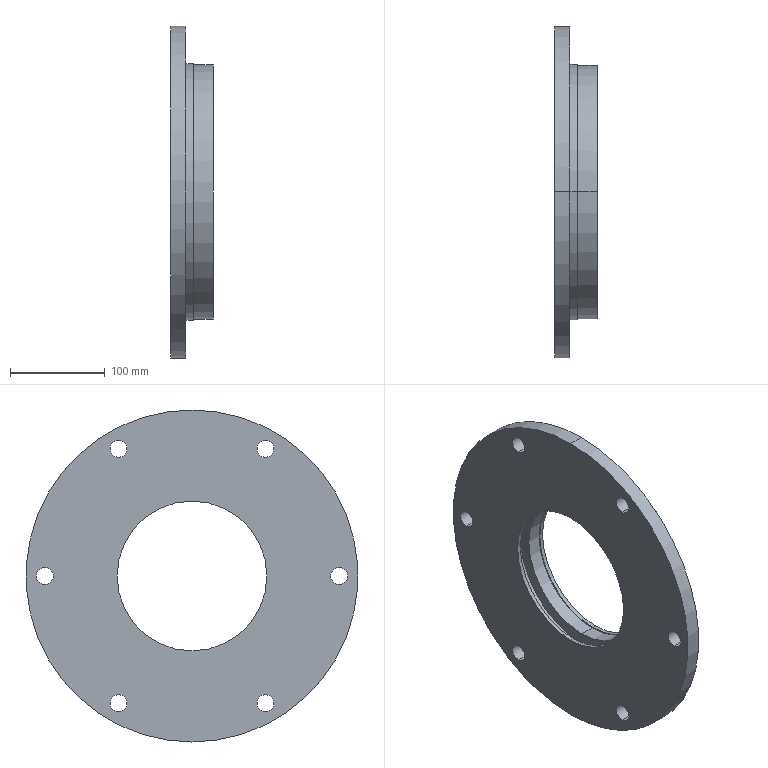Part | NX | features BREP 1 | 1 solid | 47 faces | box 45 x 350 x 350 mm | volume 1918152 mm3 | cylinder 34 | plane 9 | cone 4 | commonest cylinder face diameters 18 x12 158 x6 162 x2 176 x2 180 x2 199 x2
STEP:
#1=CARTESIAN_POINT('',(16.,77.5,-143.234));
#2=VERTEX_POINT('',#1);
#3=CARTESIAN_POINT('',(16.,77.5,-125.234));
#4=VERTEX_POINT('',#3);
#5=CARTESIAN_POINT('',(16.,77.5,-134.234));
#6=DIRECTION('',(-1.,0.,0.));
#7=DIRECTION('',(0.,0.,1.));
#8=AXIS2_PLACEMENT_3D('',#5,#6,#7);
#9=CIRCLE('',#8,9.);
#10=EDGE_CURVE('',#2,#4,#9,.T.);
#11=ORIENTED_EDGE('',*,*,#10,.F.);
#12=CARTESIAN_POINT('',(0.,77.5,-143.234));
#13=VERTEX_POINT('',#12);
#14=CARTESIAN_POINT('',(45.,77.5,-143.234));
#15=DIRECTION('',(-1.,0.,0.));
#16=VECTOR('',#15,1000.);
#17=LINE('',#14,#16);
#18=EDGE_CURVE('',#2,#13,#17,.T.);
#19=ORIENTED_EDGE('',*,*,#18,.T.);
#20=CARTESIAN_POINT('',(0.,77.5,-125.234));
#21=VERTEX_POINT('',#20);
#22=CARTESIAN_POINT('',(0.,77.5,-134.234));
#23=DIRECTION('',(-1.,0.,0.));
#24=DIRECTION('',(0.,0.866,0.5));
#25=AXIS2_PLACEMENT_3D('',#22,#23,#24);
#26=CIRCLE('',#25,9.);
#27=EDGE_CURVE('',#13,#21,#26,.T.);
#28=ORIENTED_EDGE('',*,*,#27,.T.);
#29=CARTESIAN_POINT('',(45.,77.5,-125.234));
#30=DIRECTION('',(-1.,0.,0.));
#31=VECTOR('',#30,1000.);
#32=LINE('',#29,#31);
#33=EDGE_CURVE('',#4,#21,#32,.T.);
#34=ORIENTED_EDGE('',*,*,#33,.F.);
#35=EDGE_LOOP('',(#11,#19,#28,#34));
#36=FACE_BOUND('',#35,.T.);
#37=CARTESIAN_POINT('',(45.,77.5,-134.234));
#38=DIRECTION('',(-1.,0.,0.));
#39=DIRECTION('',(0.,0.,-1.));
#40=AXIS2_PLACEMENT_3D('',#37,#38,#39);
#41=CYLINDRICAL_SURFACE('',#40,9.);
#42=ADVANCED_FACE('',(#36),#41,.F.);
#43=CARTESIAN_POINT('',(16.,-77.5,-143.234));
#44=VERTEX_POINT('',#43);
#45=CARTESIAN_POINT('',(16.,-77.5,-125.234));
#46=VERTEX_POINT('',#45);
#47=CARTESIAN_POINT('',(16.,-77.5,-134.234));
#48=DIRECTION('',(-1.,0.,0.));
#49=DIRECTION('',(0.,0.,1.));
#50=AXIS2_PLACEMENT_3D('',#47,#48,#49);
#51=CIRCLE('',#50,9.);
#52=EDGE_CURVE('',#44,#46,#51,.T.);
#53=ORIENTED_EDGE('',*,*,#52,.F.);
#54=CARTESIAN_POINT('',(0.,-77.5,-143.234));
#55=VERTEX_POINT('',#54);
#56=CARTESIAN_POINT('',(45.,-77.5,-143.234));
#57=DIRECTION('',(-1.,0.,0.));
#58=VECTOR('',#57,1000.);
#59=LINE('',#56,#58);
#60=EDGE_CURVE('',#44,#55,#59,.T.);
#61=ORIENTED_EDGE('',*,*,#60,.T.);
#62=CARTESIAN_POINT('',(0.,-77.5,-125.234));
#63=VERTEX_POINT('',#62);
#64=CARTESIAN_POINT('',(0.,-77.5,-134.234));
#65=DIRECTION('',(-1.,0.,0.));
#66=DIRECTION('',(0.,0.866,-0.5));
#67=AXIS2_PLACEMENT_3D('',#64,#65,#66);
#68=CIRCLE('',#67,9.);
#69=EDGE_CURVE('',#55,#63,#68,.T.);
#70=ORIENTED_EDGE('',*,*,#69,.T.);
#71=CARTESIAN_POINT('',(45.,-77.5,-125.234));
#72=DIRECTION('',(-1.,0.,0.));
#73=VECTOR('',#72,1000.);
#74=LINE('',#71,#73);
#75=EDGE_CURVE('',#46,#63,#74,.T.);
#76=ORIENTED_EDGE('',*,*,#75,.F.);
#77=EDGE_LOOP('',(#53,#61,#70,#76));
#78=FACE_BOUND('',#77,.T.);
#79=CARTESIAN_POINT('',(45.,-77.5,-134.234));
#80=DIRECTION('',(-1.,0.,0.));
#81=DIRECTION('',(0.,0.,-1.));
#82=AXIS2_PLACEMENT_3D('',#79,#80,#81);
#83=CYLINDRICAL_SURFACE('',#82,9.);
#84=ADVANCED_FACE('',(#78),#83,.F.);
#85=CARTESIAN_POINT('',(16.,-155.,-9.));
#86=VERTEX_POINT('',#85);
#87=CARTESIAN_POINT('',(16.,-155.,9.));
#88=VERTEX_POINT('',#87);
#89=CARTESIAN_POINT('',(16.,-155.,0.));
#90=DIRECTION('',(-1.,0.,0.));
#91=DIRECTION('',(0.,0.,1.));
#92=AXIS2_PLACEMENT_3D('',#89,#90,#91);
#93=CIRCLE('',#92,9.);
#94=EDGE_CURVE('',#86,#88,#93,.T.);
#95=ORIENTED_EDGE('',*,*,#94,.F.);
#96=CARTESIAN_POINT('',(0.,-155.,-9.));
#97=VERTEX_POINT('',#96);
#98=CARTESIAN_POINT('',(45.,-155.,-9.));
#99=DIRECTION('',(-1.,0.,0.));
#100=VECTOR('',#99,1000.);
#101=LINE('',#98,#100);
#102=EDGE_CURVE('',#86,#97,#101,.T.);
#103=ORIENTED_EDGE('',*,*,#102,.T.);
#104=CARTESIAN_POINT('',(0.,-155.,9.));
#105=VERTEX_POINT('',#104);
#106=CARTESIAN_POINT('',(0.,-155.,0.));
#107=DIRECTION('',(-1.,0.,0.));
#108=DIRECTION('',(0.,0.,-1.));
#109=AXIS2_PLACEMENT_3D('',#106,#107,#108);
#110=CIRCLE('',#109,9.);
#111=EDGE_CURVE('',#97,#105,#110,.T.);
#112=ORIENTED_EDGE('',*,*,#111,.T.);
#113=CARTESIAN_POINT('',(45.,-155.,9.));
#114=DIRECTION('',(-1.,0.,0.));
#115=VECTOR('',#114,1000.);
#116=LINE('',#113,#115);
#117=EDGE_CURVE('',#88,#105,#116,.T.);
#118=ORIENTED_EDGE('',*,*,#117,.F.);
#119=EDGE_LOOP('',(#95,#103,#112,#118));
#120=FACE_BOUND('',#119,.T.);
#121=CARTESIAN_POINT('',(45.,-155.,0.));
#122=DIRECTION('',(-1.,0.,0.));
#123=DIRECTION('',(0.,0.,-1.));
#124=AXIS2_PLACEMENT_3D('',#121,#122,#123);
#125=CYLINDRICAL_SURFACE('',#124,9.);
#126=ADVANCED_FACE('',(#120),#125,.F.);
#127=CARTESIAN_POINT('',(16.,-77.5,125.234));
#128=VERTEX_POINT('',#127);
#129=CARTESIAN_POINT('',(16.,-77.5,143.234));
#130=VERTEX_POINT('',#129);
#131=CARTESIAN_POINT('',(16.,-77.5,134.234));
#132=DIRECTION('',(-1.,0.,0.));
#133=DIRECTION('',(0.,0.,1.));
#134=AXIS2_PLACEMENT_3D('',#131,#132,#133);
#135=CIRCLE('',#134,9.);
#136=EDGE_CURVE('',#128,#130,#135,.T.);
#137=ORIENTED_EDGE('',*,*,#136,.F.);
#138=CARTESIAN_POINT('',(0.,-77.5,125.234));
#139=VERTEX_POINT('',#138);
#140=CARTESIAN_POINT('',(45.,-77.5,125.234));
#141=DIRECTION('',(-1.,0.,0.));
#142=VECTOR('',#141,1000.);
#143=LINE('',#140,#142);
#144=EDGE_CURVE('',#128,#139,#143,.T.);
#145=ORIENTED_EDGE('',*,*,#144,.T.);
#146=CARTESIAN_POINT('',(0.,-77.5,143.234));
#147=VERTEX_POINT('',#146);
#148=CARTESIAN_POINT('',(0.,-77.5,134.234));
#149=DIRECTION('',(-1.,0.,0.));
#150=DIRECTION('',(0.,-0.866,-0.5));
#151=AXIS2_PLACEMENT_3D('',#148,#149,#150);
#152=CIRCLE('',#151,9.);
#153=EDGE_CURVE('',#139,#147,#152,.T.);
#154=ORIENTED_EDGE('',*,*,#153,.T.);
#155=CARTESIAN_POINT('',(45.,-77.5,143.234));
#156=DIRECTION('',(-1.,0.,0.));
#157=VECTOR('',#156,1000.);
#158=LINE('',#155,#157);
#159=EDGE_CURVE('',#130,#147,#158,.T.);
#160=ORIENTED_EDGE('',*,*,#159,.F.);
#161=EDGE_LOOP('',(#137,#145,#154,#160));
#162=FACE_BOUND('',#161,.T.);
#163=CARTESIAN_POINT('',(45.,-77.5,134.234));
#164=DIRECTION('',(-1.,0.,0.));
#165=DIRECTION('',(0.,0.,-1.));
#166=AXIS2_PLACEMENT_3D('',#163,#164,#165);
#167=CYLINDRICAL_SURFACE('',#166,9.);
#168=ADVANCED_FACE('',(#162),#167,.F.);
#169=CARTESIAN_POINT('',(16.,77.5,125.234));
#170=VERTEX_POINT('',#169);
#171=CARTESIAN_POINT('',(16.,77.5,143.234));
#172=VERTEX_POINT('',#171);
#173=CARTESIAN_POINT('',(16.,77.5,134.234));
#174=DIRECTION('',(-1.,0.,0.));
#175=DIRECTION('',(0.,0.,1.));
#176=AXIS2_PLACEMENT_3D('',#173,#174,#175);
#177=CIRCLE('',#176,9.);
#178=EDGE_CURVE('',#170,#172,#177,.T.);
#179=ORIENTED_EDGE('',*,*,#178,.F.);
#180=CARTESIAN_POINT('',(0.,77.5,125.234));
#181=VERTEX_POINT('',#180);
#182=CARTESIAN_POINT('',(45.,77.5,125.234));
#183=DIRECTION('',(-1.,0.,0.));
#184=VECTOR('',#183,1000.);
#185=LINE('',#182,#184);
#186=EDGE_CURVE('',#170,#181,#185,.T.);
#187=ORIENTED_EDGE('',*,*,#186,.T.);
#188=CARTESIAN_POINT('',(0.,77.5,143.234));
#189=VERTEX_POINT('',#188);
#190=CARTESIAN_POINT('',(0.,77.5,134.234));
#191=DIRECTION('',(-1.,0.,0.));
#192=DIRECTION('',(0.,-0.866,0.5));
#193=AXIS2_PLACEMENT_3D('',#190,#191,#192);
#194=CIRCLE('',#193,9.);
#195=EDGE_CURVE('',#181,#189,#194,.T.);
#196=ORIENTED_EDGE('',*,*,#195,.T.);
#197=CARTESIAN_POINT('',(45.,77.5,143.234));
#198=DIRECTION('',(-1.,0.,0.));
#199=VECTOR('',#198,1000.);
#200=LINE('',#197,#199);
#201=EDGE_CURVE('',#172,#189,#200,.T.);
#202=ORIENTED_EDGE('',*,*,#201,.F.);
#203=EDGE_LOOP('',(#179,#187,#196,#202));
#204=FACE_BOUND('',#203,.T.);
#205=CARTESIAN_POINT('',(45.,77.5,134.234));
#206=DIRECTION('',(-1.,0.,0.));
#207=DIRECTION('',(0.,0.,-1.));
#208=AXIS2_PLACEMENT_3D('',#205,#206,#207);
#209=CYLINDRICAL_SURFACE('',#208,9.);
#210=ADVANCED_FACE('',(#204),#209,.F.);
#211=CARTESIAN_POINT('',(16.,155.,-9.));
#212=VERTEX_POINT('',#211);
#213=CARTESIAN_POINT('',(16.,155.,9.));
#214=VERTEX_POINT('',#213);
#215=CARTESIAN_POINT('',(16.,155.,0.));
#216=DIRECTION('',(-1.,0.,0.));
#217=DIRECTION('',(0.,0.,1.));
#218=AXIS2_PLACEMENT_3D('',#215,#216,#217);
#219=CIRCLE('',#218,9.);
#220=EDGE_CURVE('',#212,#214,#219,.T.);
#221=ORIENTED_EDGE('',*,*,#220,.F.);
#222=CARTESIAN_POINT('',(0.,155.,-9.));
#223=VERTEX_POINT('',#222);
#224=CARTESIAN_POINT('',(45.,155.,-9.));
#225=DIRECTION('',(-1.,0.,0.));
#226=VECTOR('',#225,1000.);
#227=LINE('',#224,#226);
#228=EDGE_CURVE('',#212,#223,#227,.T.);
#229=ORIENTED_EDGE('',*,*,#228,.T.);
#230=CARTESIAN_POINT('',(0.,155.,9.));
#231=VERTEX_POINT('',#230);
#232=CARTESIAN_POINT('',(0.,155.,0.));
#233=DIRECTION('',(-1.,0.,0.));
#234=DIRECTION('',(0.,0.,1.));
#235=AXIS2_PLACEMENT_3D('',#232,#233,#234);
#236=CIRCLE('',#235,9.);
#237=EDGE_CURVE('',#223,#231,#236,.T.);
#238=ORIENTED_EDGE('',*,*,#237,.T.);
#239=CARTESIAN_POINT('',(45.,155.,9.));
#240=DIRECTION('',(-1.,0.,0.));
#241=VECTOR('',#240,1000.);
#242=LINE('',#239,#241);
#243=EDGE_CURVE('',#214,#231,#242,.T.);
#244=ORIENTED_EDGE('',*,*,#243,.F.);
#245=EDGE_LOOP('',(#221,#229,#238,#244));
#246=FACE_BOUND('',#245,.T.);
#247=CARTESIAN_POINT('',(45.,155.,0.));
#248=DIRECTION('',(-1.,0.,0.));
#249=DIRECTION('',(0.,0.,-1.));
#250=AXIS2_PLACEMENT_3D('',#247,#248,#249);
#251=CYLINDRICAL_SURFACE('',#250,9.);
#252=ADVANCED_FACE('',(#246),#251,.F.);
#253=CARTESIAN_POINT('',(4.,0.,-79.));
#254=VERTEX_POINT('',#253);
#255=CARTESIAN_POINT('',(4.,0.,79.));
#256=VERTEX_POINT('',#255);
#257=CARTESIAN_POINT('',(4.,0.,0.));
#258=DIRECTION('',(-1.,0.,0.));
#259=DIRECTION('',(0.,0.,1.));
#260=AXIS2_PLACEMENT_3D('',#257,#258,#259);
#261=CIRCLE('',#260,79.);
#262=EDGE_CURVE('',#254,#256,#261,.T.);
#263=ORIENTED_EDGE('',*,*,#262,.T.);
#264=CARTESIAN_POINT('',(5.351,0.,90.));
#265=VERTEX_POINT('',#264);
#266=CARTESIAN_POINT('',(4.,0.,79.));
#267=DIRECTION('',(0.1219,0.,0.9925));
#268=VECTOR('',#267,1000.);
#269=LINE('',#266,#268);
#270=EDGE_CURVE('',#265,#256,#269,.F.);
#271=ORIENTED_EDGE('',*,*,#270,.F.);
#272=CARTESIAN_POINT('',(5.351,0.,-90.));
#273=VERTEX_POINT('',#272);
#274=CARTESIAN_POINT('',(5.351,0.,0.));
#275=DIRECTION('',(-1.,0.,0.));
#276=DIRECTION('',(0.,0.,1.));
#277=AXIS2_PLACEMENT_3D('',#274,#275,#276);
#278=CIRCLE('',#277,90.);
#279=EDGE_CURVE('',#273,#265,#278,.T.);
#280=ORIENTED_EDGE('',*,*,#279,.F.);
#281=CARTESIAN_POINT('',(4.,0.,-79.));
#282=DIRECTION('',(0.1219,0.,-0.9925));
#283=VECTOR('',#282,1000.);
#284=LINE('',#281,#283);
#285=EDGE_CURVE('',#273,#254,#284,.F.);
#286=ORIENTED_EDGE('',*,*,#285,.T.);
#287=EDGE_LOOP('',(#263,#271,#280,#286));
#288=FACE_BOUND('',#287,.T.);
#289=CARTESIAN_POINT('',(4.,0.,0.));
#290=DIRECTION('',(1.,0.,0.));
#291=DIRECTION('',(0.,0.,1.));
#292=AXIS2_PLACEMENT_3D('',#289,#290,#291);
#293=CONICAL_SURFACE('',#292,79.,1.449);
#294=ADVANCED_FACE('',(#288),#293,.F.);
#295=CARTESIAN_POINT('',(15.351,0.,-90.));
#296=VERTEX_POINT('',#295);
#297=CARTESIAN_POINT('',(15.351,0.,90.));
#298=VERTEX_POINT('',#297);
#299=CARTESIAN_POINT('',(15.351,0.,0.));
#300=DIRECTION('',(-1.,0.,0.));
#301=DIRECTION('',(0.,0.,1.));
#302=AXIS2_PLACEMENT_3D('',#299,#300,#301);
#303=CIRCLE('',#302,90.);
#304=EDGE_CURVE('',#296,#298,#303,.T.);
#305=ORIENTED_EDGE('',*,*,#304,.F.);
#306=CARTESIAN_POINT('',(0.,0.,-90.));
#307=DIRECTION('',(-1.,0.,0.));
#308=VECTOR('',#307,1000.);
#309=LINE('',#306,#308);
#310=EDGE_CURVE('',#296,#273,#309,.T.);
#311=ORIENTED_EDGE('',*,*,#310,.T.);
#312=ORIENTED_EDGE('',*,*,#279,.T.);
#313=CARTESIAN_POINT('',(0.,0.,90.));
#314=DIRECTION('',(-1.,0.,0.));
#315=VECTOR('',#314,1000.);
#316=LINE('',#313,#315);
#317=EDGE_CURVE('',#298,#265,#316,.T.);
#318=ORIENTED_EDGE('',*,*,#317,.F.);
#319=EDGE_LOOP('',(#305,#311,#312,#318));
#320=FACE_BOUND('',#319,.T.);
#321=CARTESIAN_POINT('',(0.,0.,0.));
#322=DIRECTION('',(-1.,0.,0.));
#323=DIRECTION('',(0.,0.,-1.));
#324=AXIS2_PLACEMENT_3D('',#321,#322,#323);
#325=CYLINDRICAL_SURFACE('',#324,90.);
#326=ADVANCED_FACE('',(#320),#325,.F.);
#327=CARTESIAN_POINT('',(16.701,0.,-79.));
#328=VERTEX_POINT('',#327);
#329=CARTESIAN_POINT('',(16.701,0.,79.));
#330=VERTEX_POINT('',#329);
#331=CARTESIAN_POINT('',(16.701,0.,0.));
#332=DIRECTION('',(-1.,0.,0.));
#333=DIRECTION('',(0.,0.,1.));
#334=AXIS2_PLACEMENT_3D('',#331,#332,#333);
#335=CIRCLE('',#334,79.);
#336=EDGE_CURVE('',#328,#330,#335,.T.);
#337=ORIENTED_EDGE('',*,*,#336,.F.);
#338=CARTESIAN_POINT('',(15.351,0.,-90.));
#339=DIRECTION('',(-0.1219,0.,-0.9925));
#340=VECTOR('',#339,1000.);
#341=LINE('',#338,#340);
#342=EDGE_CURVE('',#328,#296,#341,.T.);
#343=ORIENTED_EDGE('',*,*,#342,.T.);
#344=ORIENTED_EDGE('',*,*,#304,.T.);
#345=CARTESIAN_POINT('',(15.351,0.,90.));
#346=DIRECTION('',(-0.1219,0.,0.9925));
#347=VECTOR('',#346,1000.);
#348=LINE('',#345,#347);
#349=EDGE_CURVE('',#330,#298,#348,.T.);
#350=ORIENTED_EDGE('',*,*,#349,.F.);
#351=EDGE_LOOP('',(#337,#343,#344,#350));
#352=FACE_BOUND('',#351,.T.);
#353=CARTESIAN_POINT('',(15.351,0.,0.));
#354=DIRECTION('',(-1.,0.,0.));
#355=DIRECTION('',(0.,0.,-1.));
#356=AXIS2_PLACEMENT_3D('',#353,#354,#355);
#357=CONICAL_SURFACE('',#356,90.,1.449);
#358=ADVANCED_FACE('',(#352),#357,.F.);
#359=CARTESIAN_POINT('',(32.,0.,-79.));
#360=VERTEX_POINT('',#359);
#361=CARTESIAN_POINT('',(32.,0.,79.));
#362=VERTEX_POINT('',#361);
#363=CARTESIAN_POINT('',(32.,0.,0.));
#364=DIRECTION('',(-1.,0.,0.));
#365=DIRECTION('',(0.,0.,1.));
#366=AXIS2_PLACEMENT_3D('',#363,#364,#365);
#367=CIRCLE('',#366,79.);
#368=EDGE_CURVE('',#360,#362,#367,.T.);
#369=ORIENTED_EDGE('',*,*,#368,.F.);
#370=CARTESIAN_POINT('',(0.,0.,-79.));
#371=DIRECTION('',(-1.,0.,0.));
#372=VECTOR('',#371,1000.);
#373=LINE('',#370,#372);
#374=EDGE_CURVE('',#360,#328,#373,.T.);
#375=ORIENTED_EDGE('',*,*,#374,.T.);
#376=ORIENTED_EDGE('',*,*,#336,.T.);
#377=CARTESIAN_POINT('',(0.,0.,79.));
#378=DIRECTION('',(-1.,0.,0.));
#379=VECTOR('',#378,1000.);
#380=LINE('',#377,#379);
#381=EDGE_CURVE('',#362,#330,#380,.T.);
#382=ORIENTED_EDGE('',*,*,#381,.F.);
#383=EDGE_LOOP('',(#369,#375,#376,#382));
#384=FACE_BOUND('',#383,.T.);
#385=CARTESIAN_POINT('',(0.,0.,0.));
#386=DIRECTION('',(-1.,0.,0.));
#387=DIRECTION('',(0.,0.,-1.));
#388=AXIS2_PLACEMENT_3D('',#385,#386,#387);
#389=CYLINDRICAL_SURFACE('',#388,79.);
#390=ADVANCED_FACE('',(#384),#389,.F.);
#391=CARTESIAN_POINT('',(33.,0.,-81.));
#392=VERTEX_POINT('',#391);
#393=CARTESIAN_POINT('',(33.,0.,81.));
#394=VERTEX_POINT('',#393);
#395=CARTESIAN_POINT('',(33.,0.,0.));
#396=DIRECTION('',(-1.,0.,0.));
#397=DIRECTION('',(0.,0.,1.));
#398=AXIS2_PLACEMENT_3D('',#395,#396,#397);
#399=CIRCLE('',#398,81.);
#400=EDGE_CURVE('',#392,#394,#399,.T.);
#401=ORIENTED_EDGE('',*,*,#400,.F.);
#402=CARTESIAN_POINT('',(32.,0.,-81.));
#403=VERTEX_POINT('',#402);
#404=CARTESIAN_POINT('',(0.,0.,-81.));
#405=DIRECTION('',(-1.,0.,0.));
#406=VECTOR('',#405,1000.);
#407=LINE('',#404,#406);
#408=EDGE_CURVE('',#392,#403,#407,.T.);
#409=ORIENTED_EDGE('',*,*,#408,.T.);
#410=CARTESIAN_POINT('',(32.,0.,81.));
#411=VERTEX_POINT('',#410);
#412=CARTESIAN_POINT('',(32.,0.,0.));
#413=DIRECTION('',(-1.,0.,0.));
#414=DIRECTION('',(0.,0.,1.));
#415=AXIS2_PLACEMENT_3D('',#412,#413,#414);
#416=CIRCLE('',#415,81.);
#417=EDGE_CURVE('',#403,#411,#416,.T.);
#418=ORIENTED_EDGE('',*,*,#417,.T.);
#419=CARTESIAN_POINT('',(0.,0.,81.));
#420=DIRECTION('',(-1.,0.,0.));
#421=VECTOR('',#420,1000.);
#422=LINE('',#419,#421);
#423=EDGE_CURVE('',#394,#411,#422,.T.);
#424=ORIENTED_EDGE('',*,*,#423,.F.);
#425=EDGE_LOOP('',(#401,#409,#418,#424));
#426=FACE_BOUND('',#425,.T.);
#427=CARTESIAN_POINT('',(0.,0.,0.));
#428=DIRECTION('',(-1.,0.,0.));
#429=DIRECTION('',(0.,0.,-1.));
#430=AXIS2_PLACEMENT_3D('',#427,#428,#429);
#431=CYLINDRICAL_SURFACE('',#430,81.);
#432=ADVANCED_FACE('',(#426),#431,.F.);
#433=CARTESIAN_POINT('',(37.,0.,-79.));
#434=VERTEX_POINT('',#433);
#435=CARTESIAN_POINT('',(37.,0.,79.));
#436=VERTEX_POINT('',#435);
#437=CARTESIAN_POINT('',(37.,0.,0.));
#438=DIRECTION('',(-1.,0.,0.));
#439=DIRECTION('',(0.,0.,1.));
#440=AXIS2_PLACEMENT_3D('',#437,#438,#439);
#441=CIRCLE('',#440,79.);
#442=EDGE_CURVE('',#434,#436,#441,.T.);
#443=ORIENTED_EDGE('',*,*,#442,.F.);
#444=CARTESIAN_POINT('',(33.,0.,-79.));
#445=VERTEX_POINT('',#444);
#446=CARTESIAN_POINT('',(0.,0.,-79.));
#447=DIRECTION('',(-1.,0.,0.));
#448=VECTOR('',#447,1000.);
#449=LINE('',#446,#448);
#450=EDGE_CURVE('',#434,#445,#449,.T.);
#451=ORIENTED_EDGE('',*,*,#450,.T.);
#452=CARTESIAN_POINT('',(33.,0.,79.));
#453=VERTEX_POINT('',#452);
#454=CARTESIAN_POINT('',(33.,0.,0.));
#455=DIRECTION('',(-1.,0.,0.));
#456=DIRECTION('',(0.,0.,1.));
#457=AXIS2_PLACEMENT_3D('',#454,#455,#456);
#458=CIRCLE('',#457,79.);
#459=EDGE_CURVE('',#445,#453,#458,.T.);
#460=ORIENTED_EDGE('',*,*,#459,.T.);
#461=CARTESIAN_POINT('',(0.,0.,79.));
#462=DIRECTION('',(-1.,0.,0.));
#463=VECTOR('',#462,1000.);
#464=LINE('',#461,#463);
#465=EDGE_CURVE('',#436,#453,#464,.T.);
#466=ORIENTED_EDGE('',*,*,#465,.F.);
#467=EDGE_LOOP('',(#443,#451,#460,#466));
#468=FACE_BOUND('',#467,.T.);
#469=CARTESIAN_POINT('',(0.,0.,0.));
#470=DIRECTION('',(-1.,0.,0.));
#471=DIRECTION('',(0.,0.,-1.));
#472=AXIS2_PLACEMENT_3D('',#469,#470,#471);
#473=CYLINDRICAL_SURFACE('',#472,79.);
#474=ADVANCED_FACE('',(#468),#473,.F.);
#475=CARTESIAN_POINT('',(37.,0.,88.));
#476=VERTEX_POINT('',#475);
#477=CARTESIAN_POINT('',(37.,0.,-88.));
#478=VERTEX_POINT('',#477);
#479=CARTESIAN_POINT('',(37.,0.,0.));
#480=DIRECTION('',(-1.,0.,0.));
#481=DIRECTION('',(0.,0.,1.));
#482=AXIS2_PLACEMENT_3D('',#479,#480,#481);
#483=CIRCLE('',#482,88.);
#484=EDGE_CURVE('',#476,#478,#483,.T.);
#485=ORIENTED_EDGE('',*,*,#484,.T.);
#486=CARTESIAN_POINT('',(29.,0.,-88.));
#487=VERTEX_POINT('',#486);
#488=CARTESIAN_POINT('',(0.,0.,-88.));
#489=DIRECTION('',(-1.,0.,0.));
#490=VECTOR('',#489,1000.);
#491=LINE('',#488,#490);
#492=EDGE_CURVE('',#478,#487,#491,.T.);
#493=ORIENTED_EDGE('',*,*,#492,.T.);
#494=CARTESIAN_POINT('',(29.,0.,88.));
#495=VERTEX_POINT('',#494);
#496=CARTESIAN_POINT('',(29.,0.,0.));
#497=DIRECTION('',(-1.,0.,0.));
#498=DIRECTION('',(0.,0.,1.));
#499=AXIS2_PLACEMENT_3D('',#496,#497,#498);
#500=CIRCLE('',#499,88.);
#501=EDGE_CURVE('',#495,#487,#500,.T.);
#502=ORIENTED_EDGE('',*,*,#501,.F.);
#503=CARTESIAN_POINT('',(0.,0.,88.));
#504=DIRECTION('',(-1.,0.,0.));
#505=VECTOR('',#504,1000.);
#506=LINE('',#503,#505);
#507=EDGE_CURVE('',#476,#495,#506,.T.);
#508=ORIENTED_EDGE('',*,*,#507,.F.);
#509=EDGE_LOOP('',(#485,#493,#502,#508));
#510=FACE_BOUND('',#509,.T.);
#511=CARTESIAN_POINT('',(0.,0.,0.));
#512=DIRECTION('',(-1.,0.,0.));
#513=DIRECTION('',(0.,0.,-1.));
#514=AXIS2_PLACEMENT_3D('',#511,#512,#513);
#515=CYLINDRICAL_SURFACE('',#514,88.);
#516=ADVANCED_FACE('',(#510),#515,.T.);
#517=CARTESIAN_POINT('',(37.,0.,-99.5));
#518=VERTEX_POINT('',#517);
#519=CARTESIAN_POINT('',(37.,0.,99.5));
#520=VERTEX_POINT('',#519);
#521=CARTESIAN_POINT('',(37.,0.,0.));
#522=DIRECTION('',(-1.,0.,0.));
#523=DIRECTION('',(0.,0.,1.));
#524=AXIS2_PLACEMENT_3D('',#521,#522,#523);
#525=CIRCLE('',#524,99.5);
#526=EDGE_CURVE('',#518,#520,#525,.T.);
#527=ORIENTED_EDGE('',*,*,#526,.F.);
#528=CARTESIAN_POINT('',(29.,0.,-99.5));
#529=VERTEX_POINT('',#528);
#530=CARTESIAN_POINT('',(0.,0.,-99.5));
#531=DIRECTION('',(-1.,0.,0.));
#532=VECTOR('',#531,1000.);
#533=LINE('',#530,#532);
#534=EDGE_CURVE('',#518,#529,#533,.T.);
#535=ORIENTED_EDGE('',*,*,#534,.T.);
#536=CARTESIAN_POINT('',(29.,0.,99.5));
#537=VERTEX_POINT('',#536);
#538=CARTESIAN_POINT('',(29.,0.,0.));
#539=DIRECTION('',(-1.,0.,0.));
#540=DIRECTION('',(0.,0.,1.));
#541=AXIS2_PLACEMENT_3D('',#538,#539,#540);
#542=CIRCLE('',#541,99.5);
#543=EDGE_CURVE('',#529,#537,#542,.T.);
#544=ORIENTED_EDGE('',*,*,#543,.T.);
#545=CARTESIAN_POINT('',(0.,0.,99.5));
#546=DIRECTION('',(-1.,0.,0.));
#547=VECTOR('',#546,1000.);
#548=LINE('',#545,#547);
#549=EDGE_CURVE('',#520,#537,#548,.T.);
#550=ORIENTED_EDGE('',*,*,#549,.F.);
#551=EDGE_LOOP('',(#527,#535,#544,#550));
#552=FACE_BOUND('',#551,.T.);
#553=CARTESIAN_POINT('',(0.,0.,0.));
#554=DIRECTION('',(-1.,0.,0.));
#555=DIRECTION('',(0.,0.,-1.));
#556=AXIS2_PLACEMENT_3D('',#553,#554,#555);
#557=CYLINDRICAL_SURFACE('',#556,99.5);
#558=ADVANCED_FACE('',(#552),#557,.F.);
#559=CARTESIAN_POINT('',(45.,0.,-125.));
#560=VERTEX_POINT('',#559);
#561=CARTESIAN_POINT('',(45.,0.,125.));
#562=VERTEX_POINT('',#561);
#563=CARTESIAN_POINT('',(45.,0.,0.));
#564=DIRECTION('',(-1.,0.,0.));
#565=DIRECTION('',(0.,0.,1.));
#566=AXIS2_PLACEMENT_3D('',#563,#564,#565);
#567=CIRCLE('',#566,125.);
#568=EDGE_CURVE('',#560,#562,#567,.T.);
#569=ORIENTED_EDGE('',*,*,#568,.F.);
#570=CARTESIAN_POINT('',(37.,0.,-125.));
#571=VERTEX_POINT('',#570);
#572=CARTESIAN_POINT('',(0.,0.,-125.));
#573=DIRECTION('',(-1.,0.,0.));
#574=VECTOR('',#573,1000.);
#575=LINE('',#572,#574);
#576=EDGE_CURVE('',#560,#571,#575,.T.);
#577=ORIENTED_EDGE('',*,*,#576,.T.);
#578=CARTESIAN_POINT('',(37.,0.,125.));
#579=VERTEX_POINT('',#578);
#580=CARTESIAN_POINT('',(37.,0.,0.));
#581=DIRECTION('',(-1.,0.,0.));
#582=DIRECTION('',(0.,0.,1.));
#583=AXIS2_PLACEMENT_3D('',#580,#581,#582);
#584=CIRCLE('',#583,125.);
#585=EDGE_CURVE('',#571,#579,#584,.T.);
#586=ORIENTED_EDGE('',*,*,#585,.T.);
#587=CARTESIAN_POINT('',(0.,0.,125.));
#588=DIRECTION('',(-1.,0.,0.));
#589=VECTOR('',#588,1000.);
#590=LINE('',#587,#589);
#591=EDGE_CURVE('',#562,#579,#590,.T.);
#592=ORIENTED_EDGE('',*,*,#591,.F.);
#593=EDGE_LOOP('',(#569,#577,#586,#592));
#594=FACE_BOUND('',#593,.T.);
#595=CARTESIAN_POINT('',(0.,0.,0.));
#596=DIRECTION('',(-1.,0.,0.));
#597=DIRECTION('',(0.,0.,-1.));
#598=AXIS2_PLACEMENT_3D('',#595,#596,#597);
#599=CYLINDRICAL_SURFACE('',#598,125.);
#600=ADVANCED_FACE('',(#594),#599,.F.);
#601=CARTESIAN_POINT('',(45.,0.,134.));
#602=VERTEX_POINT('',#601);
#603=CARTESIAN_POINT('',(45.,0.,-134.));
#604=VERTEX_POINT('',#603);
#605=CARTESIAN_POINT('',(45.,0.,0.));
#606=DIRECTION('',(-1.,0.,0.));
#607=DIRECTION('',(0.,0.,1.));
#608=AXIS2_PLACEMENT_3D('',#605,#606,#607);
#609=CIRCLE('',#608,134.);
#610=EDGE_CURVE('',#602,#604,#609,.T.);
#611=ORIENTED_EDGE('',*,*,#610,.T.);
#612=CARTESIAN_POINT('',(24.,0.,-134.));
#613=VERTEX_POINT('',#612);
#614=CARTESIAN_POINT('',(0.,0.,-134.));
#615=DIRECTION('',(-1.,0.,0.));
#616=VECTOR('',#615,1000.);
#617=LINE('',#614,#616);
#618=EDGE_CURVE('',#604,#613,#617,.T.);
#619=ORIENTED_EDGE('',*,*,#618,.T.);
#620=CARTESIAN_POINT('',(24.,0.,134.));
#621=VERTEX_POINT('',#620);
#622=CARTESIAN_POINT('',(24.,0.,0.));
#623=DIRECTION('',(-1.,0.,0.));
#624=DIRECTION('',(0.,0.,1.));
#625=AXIS2_PLACEMENT_3D('',#622,#623,#624);
#626=CIRCLE('',#625,134.);
#627=EDGE_CURVE('',#621,#613,#626,.T.);
#628=ORIENTED_EDGE('',*,*,#627,.F.);
#629=CARTESIAN_POINT('',(0.,0.,134.));
#630=DIRECTION('',(-1.,0.,0.));
#631=VECTOR('',#630,1000.);
#632=LINE('',#629,#631);
#633=EDGE_CURVE('',#602,#621,#632,.T.);
#634=ORIENTED_EDGE('',*,*,#633,.F.);
#635=EDGE_LOOP('',(#611,#619,#628,#634));
#636=FACE_BOUND('',#635,.T.);
#637=CARTESIAN_POINT('',(0.,0.,0.));
#638=DIRECTION('',(-1.,0.,0.));
#639=DIRECTION('',(0.,0.,-1.));
#640=AXIS2_PLACEMENT_3D('',#637,#638,#639);
#641=CYLINDRICAL_SURFACE('',#640,134.);
#642=ADVANCED_FACE('',(#636),#641,.T.);
#643=CARTESIAN_POINT('',(24.,0.,135.));
#644=VERTEX_POINT('',#643);
#645=CARTESIAN_POINT('',(24.,0.,-135.));
#646=VERTEX_POINT('',#645);
#647=CARTESIAN_POINT('',(24.,0.,0.));
#648=DIRECTION('',(-1.,0.,0.));
#649=DIRECTION('',(0.,0.,1.));
#650=AXIS2_PLACEMENT_3D('',#647,#648,#649);
#651=CIRCLE('',#650,135.);
#652=EDGE_CURVE('',#644,#646,#651,.T.);
#653=ORIENTED_EDGE('',*,*,#652,.T.);
#654=CARTESIAN_POINT('',(16.,0.,-135.));
#655=VERTEX_POINT('',#654);
#656=CARTESIAN_POINT('',(0.,0.,-135.));
#657=DIRECTION('',(-1.,0.,0.));
#658=VECTOR('',#657,1000.);
#659=LINE('',#656,#658);
#660=EDGE_CURVE('',#646,#655,#659,.T.);
#661=ORIENTED_EDGE('',*,*,#660,.T.);
#662=CARTESIAN_POINT('',(16.,0.,135.));
#663=VERTEX_POINT('',#662);
#664=CARTESIAN_POINT('',(16.,0.,0.));
#665=DIRECTION('',(-1.,0.,0.));
#666=DIRECTION('',(0.,0.,1.));
#667=AXIS2_PLACEMENT_3D('',#664,#665,#666);
#668=CIRCLE('',#667,135.);
#669=EDGE_CURVE('',#663,#655,#668,.T.);
#670=ORIENTED_EDGE('',*,*,#669,.F.);
#671=CARTESIAN_POINT('',(0.,0.,135.));
#672=DIRECTION('',(-1.,0.,0.));
#673=VECTOR('',#672,1000.);
#674=LINE('',#671,#673);
#675=EDGE_CURVE('',#644,#663,#674,.T.);
#676=ORIENTED_EDGE('',*,*,#675,.F.);
#677=EDGE_LOOP('',(#653,#661,#670,#676));
#678=FACE_BOUND('',#677,.T.);
#679=CARTESIAN_POINT('',(0.,0.,0.));
#680=DIRECTION('',(-1.,0.,0.));
#681=DIRECTION('',(0.,0.,-1.));
#682=AXIS2_PLACEMENT_3D('',#679,#680,#681);
#683=CYLINDRICAL_SURFACE('',#682,135.);
#684=ADVANCED_FACE('',(#678),#683,.T.);
#685=CARTESIAN_POINT('',(16.,0.,175.));
#686=VERTEX_POINT('',#685);
#687=CARTESIAN_POINT('',(16.,0.,-175.));
#688=VERTEX_POINT('',#687);
#689=CARTESIAN_POINT('',(16.,0.,0.));
#690=DIRECTION('',(-1.,0.,0.));
#691=DIRECTION('',(0.,0.,1.));
#692=AXIS2_PLACEMENT_3D('',#689,#690,#691);
#693=CIRCLE('',#692,175.);
#694=EDGE_CURVE('',#686,#688,#693,.T.);
#695=ORIENTED_EDGE('',*,*,#694,.T.);
#696=CARTESIAN_POINT('',(0.,0.,-175.));
#697=VERTEX_POINT('',#696);
#698=CARTESIAN_POINT('',(0.,0.,-175.));
#699=DIRECTION('',(-1.,0.,0.));
#700=VECTOR('',#699,1000.);
#701=LINE('',#698,#700);
#702=EDGE_CURVE('',#688,#697,#701,.T.);
#703=ORIENTED_EDGE('',*,*,#702,.T.);
#704=CARTESIAN_POINT('',(0.,0.,175.));
#705=VERTEX_POINT('',#704);
#706=CARTESIAN_POINT('',(0.,0.,0.));
#707=DIRECTION('',(-1.,0.,0.));
#708=DIRECTION('',(0.,0.,1.));
#709=AXIS2_PLACEMENT_3D('',#706,#707,#708);
#710=CIRCLE('',#709,175.);
#711=EDGE_CURVE('',#705,#697,#710,.T.);
#712=ORIENTED_EDGE('',*,*,#711,.F.);
#713=CARTESIAN_POINT('',(0.,0.,175.));
#714=DIRECTION('',(-1.,0.,0.));
#715=VECTOR('',#714,1000.);
#716=LINE('',#713,#715);
#717=EDGE_CURVE('',#686,#705,#716,.T.);
#718=ORIENTED_EDGE('',*,*,#717,.F.);
#719=EDGE_LOOP('',(#695,#703,#712,#718));
#720=FACE_BOUND('',#719,.T.);
#721=CARTESIAN_POINT('',(0.,0.,0.));
#722=DIRECTION('',(-1.,0.,0.));
#723=DIRECTION('',(0.,0.,-1.));
#724=AXIS2_PLACEMENT_3D('',#721,#722,#723);
#725=CYLINDRICAL_SURFACE('',#724,175.);
#726=ADVANCED_FACE('',(#720),#725,.T.);
#727=ORIENTED_EDGE('',*,*,#262,.F.);
#728=CARTESIAN_POINT('',(0.,0.,-79.));
#729=VERTEX_POINT('',#728);
#730=CARTESIAN_POINT('',(0.,0.,-79.));
#731=DIRECTION('',(-1.,0.,0.));
#732=VECTOR('',#731,1000.);
#733=LINE('',#730,#732);
#734=EDGE_CURVE('',#254,#729,#733,.T.);
#735=ORIENTED_EDGE('',*,*,#734,.T.);
#736=CARTESIAN_POINT('',(0.,0.,79.));
#737=VERTEX_POINT('',#736);
#738=CARTESIAN_POINT('',(0.,0.,0.));
#739=DIRECTION('',(-1.,0.,0.));
#740=DIRECTION('',(0.,0.,1.));
#741=AXIS2_PLACEMENT_3D('',#738,#739,#740);
#742=CIRCLE('',#741,79.);
#743=EDGE_CURVE('',#729,#737,#742,.T.);
#744=ORIENTED_EDGE('',*,*,#743,.T.);
#745=CARTESIAN_POINT('',(0.,0.,79.));
#746=DIRECTION('',(-1.,0.,0.));
#747=VECTOR('',#746,1000.);
#748=LINE('',#745,#747);
#749=EDGE_CURVE('',#256,#737,#748,.T.);
#750=ORIENTED_EDGE('',*,*,#749,.F.);
#751=EDGE_LOOP('',(#727,#735,#744,#750));
#752=FACE_BOUND('',#751,.T.);
#753=CARTESIAN_POINT('',(0.,0.,0.));
#754=DIRECTION('',(-1.,0.,0.));
#755=DIRECTION('',(0.,0.,-1.));
#756=AXIS2_PLACEMENT_3D('',#753,#754,#755);
#757=CYLINDRICAL_SURFACE('',#756,79.);
#758=ADVANCED_FACE('',(#752),#757,.F.);
#759=ORIENTED_EDGE('',*,*,#734,.F.);
#760=CARTESIAN_POINT('',(4.,0.,0.));
#761=DIRECTION('',(-1.,0.,0.));
#762=DIRECTION('',(0.,0.,1.));
#763=AXIS2_PLACEMENT_3D('',#760,#761,#762);
#764=CIRCLE('',#763,79.);
#765=EDGE_CURVE('',#256,#254,#764,.T.);
#766=ORIENTED_EDGE('',*,*,#765,.F.);
#767=ORIENTED_EDGE('',*,*,#749,.T.);
#768=CARTESIAN_POINT('',(0.,0.,0.));
#769=DIRECTION('',(-1.,0.,0.));
#770=DIRECTION('',(0.,0.,1.));
#771=AXIS2_PLACEMENT_3D('',#768,#769,#770);
#772=CIRCLE('',#771,79.);
#773=EDGE_CURVE('',#737,#729,#772,.T.);
#774=ORIENTED_EDGE('',*,*,#773,.T.);
#775=EDGE_LOOP('',(#759,#766,#767,#774));
#776=FACE_BOUND('',#775,.T.);
#777=CARTESIAN_POINT('',(0.,0.,0.));
#778=DIRECTION('',(-1.,0.,0.));
#779=DIRECTION('',(0.,0.,-1.));
#780=AXIS2_PLACEMENT_3D('',#777,#778,#779);
#781=CYLINDRICAL_SURFACE('',#780,79.);
#782=ADVANCED_FACE('',(#776),#781,.F.);
#783=CARTESIAN_POINT('',(0.,77.5,-134.234));
#784=DIRECTION('',(-1.,0.,0.));
#785=DIRECTION('',(0.,0.866,0.5));
#786=AXIS2_PLACEMENT_3D('',#783,#784,#785);
#787=CIRCLE('',#786,9.);
#788=EDGE_CURVE('',#21,#13,#787,.T.);
#789=ORIENTED_EDGE('',*,*,#788,.F.);
#790=ORIENTED_EDGE('',*,*,#27,.F.);
#791=EDGE_LOOP('',(#789,#790));
#792=FACE_BOUND('',#791,.T.);
#793=CARTESIAN_POINT('',(0.,-77.5,-134.234));
#794=DIRECTION('',(-1.,0.,0.));
#795=DIRECTION('',(0.,0.866,-0.5));
#796=AXIS2_PLACEMENT_3D('',#793,#794,#795);
#797=CIRCLE('',#796,9.);
#798=EDGE_CURVE('',#63,#55,#797,.T.);
#799=ORIENTED_EDGE('',*,*,#798,.F.);
#800=ORIENTED_EDGE('',*,*,#69,.F.);
#801=EDGE_LOOP('',(#799,#800));
#802=FACE_BOUND('',#801,.T.);
#803=CARTESIAN_POINT('',(0.,-155.,0.));
#804=DIRECTION('',(-1.,0.,0.));
#805=DIRECTION('',(0.,0.,-1.));
#806=AXIS2_PLACEMENT_3D('',#803,#804,#805);
#807=CIRCLE('',#806,9.);
#808=EDGE_CURVE('',#105,#97,#807,.T.);
#809=ORIENTED_EDGE('',*,*,#808,.F.);
#810=ORIENTED_EDGE('',*,*,#111,.F.);
#811=EDGE_LOOP('',(#809,#810));
#812=FACE_BOUND('',#811,.T.);
#813=CARTESIAN_POINT('',(0.,-77.5,134.234));
#814=DIRECTION('',(-1.,0.,0.));
#815=DIRECTION('',(0.,-0.866,-0.5));
#816=AXIS2_PLACEMENT_3D('',#813,#814,#815);
#817=CIRCLE('',#816,9.);
#818=EDGE_CURVE('',#147,#139,#817,.T.);
#819=ORIENTED_EDGE('',*,*,#818,.F.);
#820=ORIENTED_EDGE('',*,*,#153,.F.);
#821=EDGE_LOOP('',(#819,#820));
#822=FACE_BOUND('',#821,.T.);
#823=CARTESIAN_POINT('',(0.,77.5,134.234));
#824=DIRECTION('',(-1.,0.,0.));
#825=DIRECTION('',(0.,-0.866,0.5));
#826=AXIS2_PLACEMENT_3D('',#823,#824,#825);
#827=CIRCLE('',#826,9.);
#828=EDGE_CURVE('',#189,#181,#827,.T.);
#829=ORIENTED_EDGE('',*,*,#828,.F.);
#830=ORIENTED_EDGE('',*,*,#195,.F.);
#831=EDGE_LOOP('',(#829,#830));
#832=FACE_BOUND('',#831,.T.);
#833=CARTESIAN_POINT('',(0.,155.,0.));
#834=DIRECTION('',(-1.,0.,0.));
#835=DIRECTION('',(0.,0.,1.));
#836=AXIS2_PLACEMENT_3D('',#833,#834,#835);
#837=CIRCLE('',#836,9.);
#838=EDGE_CURVE('',#231,#223,#837,.T.);
#839=ORIENTED_EDGE('',*,*,#838,.F.);
#840=ORIENTED_EDGE('',*,*,#237,.F.);
#841=EDGE_LOOP('',(#839,#840));
#842=FACE_BOUND('',#841,.T.);
#843=ORIENTED_EDGE('',*,*,#773,.F.);
#844=ORIENTED_EDGE('',*,*,#743,.F.);
#845=EDGE_LOOP('',(#843,#844));
#846=FACE_BOUND('',#845,.T.);
#847=ORIENTED_EDGE('',*,*,#711,.T.);
#848=CARTESIAN_POINT('',(0.,0.,0.));
#849=DIRECTION('',(-1.,0.,0.));
#850=DIRECTION('',(0.,0.,1.));
#851=AXIS2_PLACEMENT_3D('',#848,#849,#850);
#852=CIRCLE('',#851,175.);
#853=EDGE_CURVE('',#697,#705,#852,.T.);
#854=ORIENTED_EDGE('',*,*,#853,.T.);
#855=EDGE_LOOP('',(#847,#854));
#856=FACE_BOUND('',#855,.T.);
#857=CARTESIAN_POINT('',(0.,79.,0.));
#858=DIRECTION('',(1.,0.,0.));
#859=DIRECTION('',(0.,0.,1.));
#860=AXIS2_PLACEMENT_3D('',#857,#858,#859);
#861=PLANE('',#860);
#862=ADVANCED_FACE('',(#792,#802,#812,#822,#832,#842,#846,#856),#861,.F.);
#863=ORIENTED_EDGE('',*,*,#702,.F.);
#864=CARTESIAN_POINT('',(16.,0.,0.));
#865=DIRECTION('',(-1.,0.,0.));
#866=DIRECTION('',(0.,0.,1.));
#867=AXIS2_PLACEMENT_3D('',#864,#865,#866);
#868=CIRCLE('',#867,175.);
#869=EDGE_CURVE('',#688,#686,#868,.T.);
#870=ORIENTED_EDGE('',*,*,#869,.T.);
#871=ORIENTED_EDGE('',*,*,#717,.T.);
#872=ORIENTED_EDGE('',*,*,#853,.F.);
#873=EDGE_LOOP('',(#863,#870,#871,#872));
#874=FACE_BOUND('',#873,.T.);
#875=CARTESIAN_POINT('',(0.,0.,0.));
#876=DIRECTION('',(-1.,0.,0.));
#877=DIRECTION('',(0.,0.,-1.));
#878=AXIS2_PLACEMENT_3D('',#875,#876,#877);
#879=CYLINDRICAL_SURFACE('',#878,175.);
#880=ADVANCED_FACE('',(#874),#879,.T.);
#881=CARTESIAN_POINT('',(16.,77.5,-134.234));
#882=DIRECTION('',(-1.,0.,0.));
#883=DIRECTION('',(0.,0.,1.));
#884=AXIS2_PLACEMENT_3D('',#881,#882,#883);
#885=CIRCLE('',#884,9.);
#886=EDGE_CURVE('',#4,#2,#885,.T.);
#887=ORIENTED_EDGE('',*,*,#886,.T.);
#888=ORIENTED_EDGE('',*,*,#10,.T.);
#889=EDGE_LOOP('',(#887,#888));
#890=FACE_BOUND('',#889,.T.);
#891=CARTESIAN_POINT('',(16.,-77.5,-134.234));
#892=DIRECTION('',(-1.,0.,0.));
#893=DIRECTION('',(0.,0.,1.));
#894=AXIS2_PLACEMENT_3D('',#891,#892,#893);
#895=CIRCLE('',#894,9.);
#896=EDGE_CURVE('',#46,#44,#895,.T.);
#897=ORIENTED_EDGE('',*,*,#896,.T.);
#898=ORIENTED_EDGE('',*,*,#52,.T.);
#899=EDGE_LOOP('',(#897,#898));
#900=FACE_BOUND('',#899,.T.);
#901=CARTESIAN_POINT('',(16.,-155.,0.));
#902=DIRECTION('',(-1.,0.,0.));
#903=DIRECTION('',(0.,0.,1.));
#904=AXIS2_PLACEMENT_3D('',#901,#902,#903);
#905=CIRCLE('',#904,9.);
#906=EDGE_CURVE('',#88,#86,#905,.T.);
#907=ORIENTED_EDGE('',*,*,#906,.T.);
#908=ORIENTED_EDGE('',*,*,#94,.T.);
#909=EDGE_LOOP('',(#907,#908));
#910=FACE_BOUND('',#909,.T.);
#911=CARTESIAN_POINT('',(16.,-77.5,134.234));
#912=DIRECTION('',(-1.,0.,0.));
#913=DIRECTION('',(0.,0.,1.));
#914=AXIS2_PLACEMENT_3D('',#911,#912,#913);
#915=CIRCLE('',#914,9.);
#916=EDGE_CURVE('',#130,#128,#915,.T.);
#917=ORIENTED_EDGE('',*,*,#916,.T.);
#918=ORIENTED_EDGE('',*,*,#136,.T.);
#919=EDGE_LOOP('',(#917,#918));
#920=FACE_BOUND('',#919,.T.);
#921=CARTESIAN_POINT('',(16.,77.5,134.234));
#922=DIRECTION('',(-1.,0.,0.));
#923=DIRECTION('',(0.,0.,1.));
#924=AXIS2_PLACEMENT_3D('',#921,#922,#923);
#925=CIRCLE('',#924,9.);
#926=EDGE_CURVE('',#172,#170,#925,.T.);
#927=ORIENTED_EDGE('',*,*,#926,.T.);
#928=ORIENTED_EDGE('',*,*,#178,.T.);
#929=EDGE_LOOP('',(#927,#928));
#930=FACE_BOUND('',#929,.T.);
#931=CARTESIAN_POINT('',(16.,155.,0.));
#932=DIRECTION('',(-1.,0.,0.));
#933=DIRECTION('',(0.,0.,1.));
#934=AXIS2_PLACEMENT_3D('',#931,#932,#933);
#935=CIRCLE('',#934,9.);
#936=EDGE_CURVE('',#214,#212,#935,.T.);
#937=ORIENTED_EDGE('',*,*,#936,.T.);
#938=ORIENTED_EDGE('',*,*,#220,.T.);
#939=EDGE_LOOP('',(#937,#938));
#940=FACE_BOUND('',#939,.T.);
#941=ORIENTED_EDGE('',*,*,#694,.F.);
#942=ORIENTED_EDGE('',*,*,#869,.F.);
#943=EDGE_LOOP('',(#941,#942));
#944=FACE_BOUND('',#943,.T.);
#945=ORIENTED_EDGE('',*,*,#669,.T.);
#946=CARTESIAN_POINT('',(16.,0.,0.));
#947=DIRECTION('',(-1.,0.,0.));
#948=DIRECTION('',(0.,0.,1.));
#949=AXIS2_PLACEMENT_3D('',#946,#947,#948);
#950=CIRCLE('',#949,135.);
#951=EDGE_CURVE('',#655,#663,#950,.T.);
#952=ORIENTED_EDGE('',*,*,#951,.T.);
#953=EDGE_LOOP('',(#945,#952));
#954=FACE_BOUND('',#953,.T.);
#955=CARTESIAN_POINT('',(16.,175.,0.));
#956=DIRECTION('',(-1.,0.,0.));
#957=DIRECTION('',(0.,0.,-1.));
#958=AXIS2_PLACEMENT_3D('',#955,#956,#957);
#959=PLANE('',#958);
#960=ADVANCED_FACE('',(#890,#900,#910,#920,#930,#940,#944,#954),#959,.F.);
#961=ORIENTED_EDGE('',*,*,#660,.F.);
#962=CARTESIAN_POINT('',(24.,0.,0.));
#963=DIRECTION('',(-1.,0.,0.));
#964=DIRECTION('',(0.,0.,1.));
#965=AXIS2_PLACEMENT_3D('',#962,#963,#964);
#966=CIRCLE('',#965,135.);
#967=EDGE_CURVE('',#646,#644,#966,.T.);
#968=ORIENTED_EDGE('',*,*,#967,.T.);
#969=ORIENTED_EDGE('',*,*,#675,.T.);
#970=ORIENTED_EDGE('',*,*,#951,.F.);
#971=EDGE_LOOP('',(#961,#968,#969,#970));
#972=FACE_BOUND('',#971,.T.);
#973=CARTESIAN_POINT('',(0.,0.,0.));
#974=DIRECTION('',(-1.,0.,0.));
#975=DIRECTION('',(0.,0.,-1.));
#976=AXIS2_PLACEMENT_3D('',#973,#974,#975);
#977=CYLINDRICAL_SURFACE('',#976,135.);
#978=ADVANCED_FACE('',(#972),#977,.T.);
#979=ORIENTED_EDGE('',*,*,#652,.F.);
#980=ORIENTED_EDGE('',*,*,#967,.F.);
#981=EDGE_LOOP('',(#979,#980));
#982=FACE_BOUND('',#981,.T.);
#983=ORIENTED_EDGE('',*,*,#627,.T.);
#984=CARTESIAN_POINT('',(24.,0.,0.));
#985=DIRECTION('',(-1.,0.,0.));
#986=DIRECTION('',(0.,0.,1.));
#987=AXIS2_PLACEMENT_3D('',#984,#985,#986);
#988=CIRCLE('',#987,134.);
#989=EDGE_CURVE('',#613,#621,#988,.T.);
#990=ORIENTED_EDGE('',*,*,#989,.T.);
#991=EDGE_LOOP('',(#983,#990));
#992=FACE_BOUND('',#991,.T.);
#993=CARTESIAN_POINT('',(24.,135.,0.));
#994=DIRECTION('',(-1.,0.,0.));
#995=DIRECTION('',(0.,0.,-1.));
#996=AXIS2_PLACEMENT_3D('',#993,#994,#995);
#997=PLANE('',#996);
#998=ADVANCED_FACE('',(#982,#992),#997,.F.);
#999=ORIENTED_EDGE('',*,*,#618,.F.);
#1000=CARTESIAN_POINT('',(45.,0.,0.));
#1001=DIRECTION('',(-1.,0.,0.));
#1002=DIRECTION('',(0.,0.,1.));
#1003=AXIS2_PLACEMENT_3D('',#1000,#1001,#1002);
#1004=CIRCLE('',#1003,134.);
#1005=EDGE_CURVE('',#604,#602,#1004,.T.);
#1006=ORIENTED_EDGE('',*,*,#1005,.T.);
#1007=ORIENTED_EDGE('',*,*,#633,.T.);
#1008=ORIENTED_EDGE('',*,*,#989,.F.);
#1009=EDGE_LOOP('',(#999,#1006,#1007,#1008));
#1010=FACE_BOUND('',#1009,.T.);
#1011=CARTESIAN_POINT('',(0.,0.,0.));
#1012=DIRECTION('',(-1.,0.,0.));
#1013=DIRECTION('',(0.,0.,-1.));
#1014=AXIS2_PLACEMENT_3D('',#1011,#1012,#1013);
#1015=CYLINDRICAL_SURFACE('',#1014,134.);
#1016=ADVANCED_FACE('',(#1010),#1015,.T.);
#1017=ORIENTED_EDGE('',*,*,#610,.F.);
#1018=ORIENTED_EDGE('',*,*,#1005,.F.);
#1019=EDGE_LOOP('',(#1017,#1018));
#1020=FACE_BOUND('',#1019,.T.);
#1021=CARTESIAN_POINT('',(45.,0.,0.));
#1022=DIRECTION('',(-1.,0.,0.));
#1023=DIRECTION('',(0.,0.,1.));
#1024=AXIS2_PLACEMENT_3D('',#1021,#1022,#1023);
#1025=CIRCLE('',#1024,125.);
#1026=EDGE_CURVE('',#562,#560,#1025,.T.);
#1027=ORIENTED_EDGE('',*,*,#1026,.T.);
#1028=ORIENTED_EDGE('',*,*,#568,.T.);
#1029=EDGE_LOOP('',(#1027,#1028));
#1030=FACE_BOUND('',#1029,.T.);
#1031=CARTESIAN_POINT('',(45.,134.,0.));
#1032=DIRECTION('',(-1.,0.,0.));
#1033=DIRECTION('',(0.,0.,-1.));
#1034=AXIS2_PLACEMENT_3D('',#1031,#1032,#1033);
#1035=PLANE('',#1034);
#1036=ADVANCED_FACE('',(#1020,#1030),#1035,.F.);
#1037=ORIENTED_EDGE('',*,*,#576,.F.);
#1038=ORIENTED_EDGE('',*,*,#1026,.F.);
#1039=ORIENTED_EDGE('',*,*,#591,.T.);
#1040=CARTESIAN_POINT('',(37.,0.,0.));
#1041=DIRECTION('',(-1.,0.,0.));
#1042=DIRECTION('',(0.,0.,1.));
#1043=AXIS2_PLACEMENT_3D('',#1040,#1041,#1042);
#1044=CIRCLE('',#1043,125.);
#1045=EDGE_CURVE('',#579,#571,#1044,.T.);
#1046=ORIENTED_EDGE('',*,*,#1045,.T.);
#1047=EDGE_LOOP('',(#1037,#1038,#1039,#1046));
#1048=FACE_BOUND('',#1047,.T.);
#1049=CARTESIAN_POINT('',(0.,0.,0.));
#1050=DIRECTION('',(-1.,0.,0.));
#1051=DIRECTION('',(0.,0.,-1.));
#1052=AXIS2_PLACEMENT_3D('',#1049,#1050,#1051);
#1053=CYLINDRICAL_SURFACE('',#1052,125.);
#1054=ADVANCED_FACE('',(#1048),#1053,.F.);
#1055=ORIENTED_EDGE('',*,*,#1045,.F.);
#1056=ORIENTED_EDGE('',*,*,#585,.F.);
#1057=EDGE_LOOP('',(#1055,#1056));
#1058=FACE_BOUND('',#1057,.T.);
#1059=CARTESIAN_POINT('',(37.,0.,0.));
#1060=DIRECTION('',(-1.,0.,0.));
#1061=DIRECTION('',(0.,0.,1.));
#1062=AXIS2_PLACEMENT_3D('',#1059,#1060,#1061);
#1063=CIRCLE('',#1062,99.5);
#1064=EDGE_CURVE('',#520,#518,#1063,.T.);
#1065=ORIENTED_EDGE('',*,*,#1064,.T.);
#1066=ORIENTED_EDGE('',*,*,#526,.T.);
#1067=EDGE_LOOP('',(#1065,#1066));
#1068=FACE_BOUND('',#1067,.T.);
#1069=CARTESIAN_POINT('',(37.,125.,0.));
#1070=DIRECTION('',(-1.,0.,0.));
#1071=DIRECTION('',(0.,0.,-1.));
#1072=AXIS2_PLACEMENT_3D('',#1069,#1070,#1071);
#1073=PLANE('',#1072);
#1074=ADVANCED_FACE('',(#1058,#1068),#1073,.F.);
#1075=ORIENTED_EDGE('',*,*,#534,.F.);
#1076=ORIENTED_EDGE('',*,*,#1064,.F.);
#1077=ORIENTED_EDGE('',*,*,#549,.T.);
#1078=CARTESIAN_POINT('',(29.,0.,0.));
#1079=DIRECTION('',(-1.,0.,0.));
#1080=DIRECTION('',(0.,0.,1.));
#1081=AXIS2_PLACEMENT_3D('',#1078,#1079,#1080);
#1082=CIRCLE('',#1081,99.5);
#1083=EDGE_CURVE('',#537,#529,#1082,.T.);
#1084=ORIENTED_EDGE('',*,*,#1083,.T.);
#1085=EDGE_LOOP('',(#1075,#1076,#1077,#1084));
#1086=FACE_BOUND('',#1085,.T.);
#1087=CARTESIAN_POINT('',(0.,0.,0.));
#1088=DIRECTION('',(-1.,0.,0.));
#1089=DIRECTION('',(0.,0.,-1.));
#1090=AXIS2_PLACEMENT_3D('',#1087,#1088,#1089);
#1091=CYLINDRICAL_SURFACE('',#1090,99.5);
#1092=ADVANCED_FACE('',(#1086),#1091,.F.);
#1093=ORIENTED_EDGE('',*,*,#1083,.F.);
#1094=ORIENTED_EDGE('',*,*,#543,.F.);
#1095=EDGE_LOOP('',(#1093,#1094));
#1096=FACE_BOUND('',#1095,.T.);
#1097=ORIENTED_EDGE('',*,*,#501,.T.);
#1098=CARTESIAN_POINT('',(29.,0.,0.));
#1099=DIRECTION('',(-1.,0.,0.));
#1100=DIRECTION('',(0.,0.,1.));
#1101=AXIS2_PLACEMENT_3D('',#1098,#1099,#1100);
#1102=CIRCLE('',#1101,88.);
#1103=EDGE_CURVE('',#487,#495,#1102,.T.);
#1104=ORIENTED_EDGE('',*,*,#1103,.T.);
#1105=EDGE_LOOP('',(#1097,#1104));
#1106=FACE_BOUND('',#1105,.T.);
#1107=CARTESIAN_POINT('',(29.,99.5,0.));
#1108=DIRECTION('',(-1.,0.,0.));
#1109=DIRECTION('',(0.,0.,-1.));
#1110=AXIS2_PLACEMENT_3D('',#1107,#1108,#1109);
#1111=PLANE('',#1110);
#1112=ADVANCED_FACE('',(#1096,#1106),#1111,.F.);
#1113=ORIENTED_EDGE('',*,*,#492,.F.);
#1114=CARTESIAN_POINT('',(37.,0.,0.));
#1115=DIRECTION('',(-1.,0.,0.));
#1116=DIRECTION('',(0.,0.,1.));
#1117=AXIS2_PLACEMENT_3D('',#1114,#1115,#1116);
#1118=CIRCLE('',#1117,88.);
#1119=EDGE_CURVE('',#478,#476,#1118,.T.);
#1120=ORIENTED_EDGE('',*,*,#1119,.T.);
#1121=ORIENTED_EDGE('',*,*,#507,.T.);
#1122=ORIENTED_EDGE('',*,*,#1103,.F.);
#1123=EDGE_LOOP('',(#1113,#1120,#1121,#1122));
#1124=FACE_BOUND('',#1123,.T.);
#1125=CARTESIAN_POINT('',(0.,0.,0.));
#1126=DIRECTION('',(-1.,0.,0.));
#1127=DIRECTION('',(0.,0.,-1.));
#1128=AXIS2_PLACEMENT_3D('',#1125,#1126,#1127);
#1129=CYLINDRICAL_SURFACE('',#1128,88.);
#1130=ADVANCED_FACE('',(#1124),#1129,.T.);
#1131=ORIENTED_EDGE('',*,*,#484,.F.);
#1132=ORIENTED_EDGE('',*,*,#1119,.F.);
#1133=EDGE_LOOP('',(#1131,#1132));
#1134=FACE_BOUND('',#1133,.T.);
#1135=CARTESIAN_POINT('',(37.,0.,0.));
#1136=DIRECTION('',(-1.,0.,0.));
#1137=DIRECTION('',(0.,0.,1.));
#1138=AXIS2_PLACEMENT_3D('',#1135,#1136,#1137);
#1139=CIRCLE('',#1138,79.);
#1140=EDGE_CURVE('',#436,#434,#1139,.T.);
#1141=ORIENTED_EDGE('',*,*,#1140,.T.);
#1142=ORIENTED_EDGE('',*,*,#442,.T.);
#1143=EDGE_LOOP('',(#1141,#1142));
#1144=FACE_BOUND('',#1143,.T.);
#1145=CARTESIAN_POINT('',(37.,88.,0.));
#1146=DIRECTION('',(-1.,0.,0.));
#1147=DIRECTION('',(0.,0.,-1.));
#1148=AXIS2_PLACEMENT_3D('',#1145,#1146,#1147);
#1149=PLANE('',#1148);
#1150=ADVANCED_FACE('',(#1134,#1144),#1149,.F.);
#1151=ORIENTED_EDGE('',*,*,#450,.F.);
#1152=ORIENTED_EDGE('',*,*,#1140,.F.);
#1153=ORIENTED_EDGE('',*,*,#465,.T.);
#1154=CARTESIAN_POINT('',(33.,0.,0.));
#1155=DIRECTION('',(-1.,0.,0.));
#1156=DIRECTION('',(0.,0.,1.));
#1157=AXIS2_PLACEMENT_3D('',#1154,#1155,#1156);
#1158=CIRCLE('',#1157,79.);
#1159=EDGE_CURVE('',#453,#445,#1158,.T.);
#1160=ORIENTED_EDGE('',*,*,#1159,.T.);
#1161=EDGE_LOOP('',(#1151,#1152,#1153,#1160));
#1162=FACE_BOUND('',#1161,.T.);
#1163=CARTESIAN_POINT('',(0.,0.,0.));
#1164=DIRECTION('',(-1.,0.,0.));
#1165=DIRECTION('',(0.,0.,-1.));
#1166=AXIS2_PLACEMENT_3D('',#1163,#1164,#1165);
#1167=CYLINDRICAL_SURFACE('',#1166,79.);
#1168=ADVANCED_FACE('',(#1162),#1167,.F.);
#1169=ORIENTED_EDGE('',*,*,#1159,.F.);
#1170=ORIENTED_EDGE('',*,*,#459,.F.);
#1171=EDGE_LOOP('',(#1169,#1170));
#1172=FACE_BOUND('',#1171,.T.);
#1173=CARTESIAN_POINT('',(33.,0.,0.));
#1174=DIRECTION('',(-1.,0.,0.));
#1175=DIRECTION('',(0.,0.,1.));
#1176=AXIS2_PLACEMENT_3D('',#1173,#1174,#1175);
#1177=CIRCLE('',#1176,81.);
#1178=EDGE_CURVE('',#394,#392,#1177,.T.);
#1179=ORIENTED_EDGE('',*,*,#1178,.T.);
#1180=ORIENTED_EDGE('',*,*,#400,.T.);
#1181=EDGE_LOOP('',(#1179,#1180));
#1182=FACE_BOUND('',#1181,.T.);
#1183=CARTESIAN_POINT('',(33.,79.,0.));
#1184=DIRECTION('',(1.,0.,0.));
#1185=DIRECTION('',(0.,0.,1.));
#1186=AXIS2_PLACEMENT_3D('',#1183,#1184,#1185);
#1187=PLANE('',#1186);
#1188=ADVANCED_FACE('',(#1172,#1182),#1187,.F.);
#1189=ORIENTED_EDGE('',*,*,#408,.F.);
#1190=ORIENTED_EDGE('',*,*,#1178,.F.);
#1191=ORIENTED_EDGE('',*,*,#423,.T.);
#1192=CARTESIAN_POINT('',(32.,0.,0.));
#1193=DIRECTION('',(-1.,0.,0.));
#1194=DIRECTION('',(0.,0.,1.));
#1195=AXIS2_PLACEMENT_3D('',#1192,#1193,#1194);
#1196=CIRCLE('',#1195,81.);
#1197=EDGE_CURVE('',#411,#403,#1196,.T.);
#1198=ORIENTED_EDGE('',*,*,#1197,.T.);
#1199=EDGE_LOOP('',(#1189,#1190,#1191,#1198));
#1200=FACE_BOUND('',#1199,.T.);
#1201=CARTESIAN_POINT('',(0.,0.,0.));
#1202=DIRECTION('',(-1.,0.,0.));
#1203=DIRECTION('',(0.,0.,-1.));
#1204=AXIS2_PLACEMENT_3D('',#1201,#1202,#1203);
#1205=CYLINDRICAL_SURFACE('',#1204,81.);
#1206=ADVANCED_FACE('',(#1200),#1205,.F.);
#1207=ORIENTED_EDGE('',*,*,#1197,.F.);
#1208=ORIENTED_EDGE('',*,*,#417,.F.);
#1209=EDGE_LOOP('',(#1207,#1208));
#1210=FACE_BOUND('',#1209,.T.);
#1211=CARTESIAN_POINT('',(32.,0.,0.));
#1212=DIRECTION('',(-1.,0.,0.));
#1213=DIRECTION('',(0.,0.,1.));
#1214=AXIS2_PLACEMENT_3D('',#1211,#1212,#1213);
#1215=CIRCLE('',#1214,79.);
#1216=EDGE_CURVE('',#362,#360,#1215,.T.);
#1217=ORIENTED_EDGE('',*,*,#1216,.T.);
#1218=ORIENTED_EDGE('',*,*,#368,.T.);
#1219=EDGE_LOOP('',(#1217,#1218));
#1220=FACE_BOUND('',#1219,.T.);
#1221=CARTESIAN_POINT('',(32.,81.,0.));
#1222=DIRECTION('',(-1.,0.,0.));
#1223=DIRECTION('',(0.,0.,-1.));
#1224=AXIS2_PLACEMENT_3D('',#1221,#1222,#1223);
#1225=PLANE('',#1224);
#1226=ADVANCED_FACE('',(#1210,#1220),#1225,.F.);
#1227=ORIENTED_EDGE('',*,*,#374,.F.);
#1228=ORIENTED_EDGE('',*,*,#1216,.F.);
#1229=ORIENTED_EDGE('',*,*,#381,.T.);
#1230=CARTESIAN_POINT('',(16.701,0.,0.));
#1231=DIRECTION('',(-1.,0.,0.));
#1232=DIRECTION('',(0.,0.,1.));
#1233=AXIS2_PLACEMENT_3D('',#1230,#1231,#1232);
#1234=CIRCLE('',#1233,79.);
#1235=EDGE_CURVE('',#330,#328,#1234,.T.);
#1236=ORIENTED_EDGE('',*,*,#1235,.T.);
#1237=EDGE_LOOP('',(#1227,#1228,#1229,#1236));
#1238=FACE_BOUND('',#1237,.T.);
#1239=CARTESIAN_POINT('',(0.,0.,0.));
#1240=DIRECTION('',(-1.,0.,0.));
#1241=DIRECTION('',(0.,0.,-1.));
#1242=AXIS2_PLACEMENT_3D('',#1239,#1240,#1241);
#1243=CYLINDRICAL_SURFACE('',#1242,79.);
#1244=ADVANCED_FACE('',(#1238),#1243,.F.);
#1245=ORIENTED_EDGE('',*,*,#342,.F.);
#1246=ORIENTED_EDGE('',*,*,#1235,.F.);
#1247=ORIENTED_EDGE('',*,*,#349,.T.);
#1248=CARTESIAN_POINT('',(15.351,0.,0.));
#1249=DIRECTION('',(-1.,0.,0.));
#1250=DIRECTION('',(0.,0.,1.));
#1251=AXIS2_PLACEMENT_3D('',#1248,#1249,#1250);
#1252=CIRCLE('',#1251,90.);
#1253=EDGE_CURVE('',#298,#296,#1252,.T.);
#1254=ORIENTED_EDGE('',*,*,#1253,.T.);
#1255=EDGE_LOOP('',(#1245,#1246,#1247,#1254));
#1256=FACE_BOUND('',#1255,.T.);
#1257=CARTESIAN_POINT('',(15.351,0.,0.));
#1258=DIRECTION('',(-1.,0.,0.));
#1259=DIRECTION('',(0.,0.,-1.));
#1260=AXIS2_PLACEMENT_3D('',#1257,#1258,#1259);
#1261=CONICAL_SURFACE('',#1260,90.,1.449);
#1262=ADVANCED_FACE('',(#1256),#1261,.F.);
#1263=ORIENTED_EDGE('',*,*,#310,.F.);
#1264=ORIENTED_EDGE('',*,*,#1253,.F.);
#1265=ORIENTED_EDGE('',*,*,#317,.T.);
#1266=CARTESIAN_POINT('',(5.351,0.,0.));
#1267=DIRECTION('',(-1.,0.,0.));
#1268=DIRECTION('',(0.,0.,1.));
#1269=AXIS2_PLACEMENT_3D('',#1266,#1267,#1268);
#1270=CIRCLE('',#1269,90.);
#1271=EDGE_CURVE('',#265,#273,#1270,.T.);
#1272=ORIENTED_EDGE('',*,*,#1271,.T.);
#1273=EDGE_LOOP('',(#1263,#1264,#1265,#1272));
#1274=FACE_BOUND('',#1273,.T.);
#1275=CARTESIAN_POINT('',(0.,0.,0.));
#1276=DIRECTION('',(-1.,0.,0.));
#1277=DIRECTION('',(0.,0.,-1.));
#1278=AXIS2_PLACEMENT_3D('',#1275,#1276,#1277);
#1279=CYLINDRICAL_SURFACE('',#1278,90.);
#1280=ADVANCED_FACE('',(#1274),#1279,.F.);
#1281=ORIENTED_EDGE('',*,*,#270,.T.);
#1282=ORIENTED_EDGE('',*,*,#765,.T.);
#1283=ORIENTED_EDGE('',*,*,#285,.F.);
#1284=ORIENTED_EDGE('',*,*,#1271,.F.);
#1285=EDGE_LOOP('',(#1281,#1282,#1283,#1284));
#1286=FACE_BOUND('',#1285,.T.);
#1287=CARTESIAN_POINT('',(4.,0.,0.));
#1288=DIRECTION('',(1.,0.,0.));
#1289=DIRECTION('',(0.,0.,1.));
#1290=AXIS2_PLACEMENT_3D('',#1287,#1288,#1289);
#1291=CONICAL_SURFACE('',#1290,79.,1.449);
#1292=ADVANCED_FACE('',(#1286),#1291,.F.);
#1293=ORIENTED_EDGE('',*,*,#228,.F.);
#1294=ORIENTED_EDGE('',*,*,#936,.F.);
#1295=ORIENTED_EDGE('',*,*,#243,.T.);
#1296=ORIENTED_EDGE('',*,*,#838,.T.);
#1297=EDGE_LOOP('',(#1293,#1294,#1295,#1296));
#1298=FACE_BOUND('',#1297,.T.);
#1299=CARTESIAN_POINT('',(45.,155.,0.));
#1300=DIRECTION('',(-1.,0.,0.));
#1301=DIRECTION('',(0.,0.,-1.));
#1302=AXIS2_PLACEMENT_3D('',#1299,#1300,#1301);
#1303=CYLINDRICAL_SURFACE('',#1302,9.);
#1304=ADVANCED_FACE('',(#1298),#1303,.F.);
#1305=ORIENTED_EDGE('',*,*,#186,.F.);
#1306=ORIENTED_EDGE('',*,*,#926,.F.);
#1307=ORIENTED_EDGE('',*,*,#201,.T.);
#1308=ORIENTED_EDGE('',*,*,#828,.T.);
#1309=EDGE_LOOP('',(#1305,#1306,#1307,#1308));
#1310=FACE_BOUND('',#1309,.T.);
#1311=CARTESIAN_POINT('',(45.,77.5,134.234));
#1312=DIRECTION('',(-1.,0.,0.));
#1313=DIRECTION('',(0.,0.,-1.));
#1314=AXIS2_PLACEMENT_3D('',#1311,#1312,#1313);
#1315=CYLINDRICAL_SURFACE('',#1314,9.);
#1316=ADVANCED_FACE('',(#1310),#1315,.F.);
#1317=ORIENTED_EDGE('',*,*,#144,.F.);
#1318=ORIENTED_EDGE('',*,*,#916,.F.);
#1319=ORIENTED_EDGE('',*,*,#159,.T.);
#1320=ORIENTED_EDGE('',*,*,#818,.T.);
#1321=EDGE_LOOP('',(#1317,#1318,#1319,#1320));
#1322=FACE_BOUND('',#1321,.T.);
#1323=CARTESIAN_POINT('',(45.,-77.5,134.234));
#1324=DIRECTION('',(-1.,0.,0.));
#1325=DIRECTION('',(0.,0.,-1.));
#1326=AXIS2_PLACEMENT_3D('',#1323,#1324,#1325);
#1327=CYLINDRICAL_SURFACE('',#1326,9.);
#1328=ADVANCED_FACE('',(#1322),#1327,.F.);
#1329=ORIENTED_EDGE('',*,*,#102,.F.);
#1330=ORIENTED_EDGE('',*,*,#906,.F.);
#1331=ORIENTED_EDGE('',*,*,#117,.T.);
#1332=ORIENTED_EDGE('',*,*,#808,.T.);
#1333=EDGE_LOOP('',(#1329,#1330,#1331,#1332));
#1334=FACE_BOUND('',#1333,.T.);
#1335=CARTESIAN_POINT('',(45.,-155.,0.));
#1336=DIRECTION('',(-1.,0.,0.));
#1337=DIRECTION('',(0.,0.,-1.));
#1338=AXIS2_PLACEMENT_3D('',#1335,#1336,#1337);
#1339=CYLINDRICAL_SURFACE('',#1338,9.);
#1340=ADVANCED_FACE('',(#1334),#1339,.F.);
#1341=ORIENTED_EDGE('',*,*,#60,.F.);
#1342=ORIENTED_EDGE('',*,*,#896,.F.);
#1343=ORIENTED_EDGE('',*,*,#75,.T.);
#1344=ORIENTED_EDGE('',*,*,#798,.T.);
#1345=EDGE_LOOP('',(#1341,#1342,#1343,#1344));
#1346=FACE_BOUND('',#1345,.T.);
#1347=CARTESIAN_POINT('',(45.,-77.5,-134.234));
#1348=DIRECTION('',(-1.,0.,0.));
#1349=DIRECTION('',(0.,0.,-1.));
#1350=AXIS2_PLACEMENT_3D('',#1347,#1348,#1349);
#1351=CYLINDRICAL_SURFACE('',#1350,9.);
#1352=ADVANCED_FACE('',(#1346),#1351,.F.);
#1353=ORIENTED_EDGE('',*,*,#18,.F.);
#1354=ORIENTED_EDGE('',*,*,#886,.F.);
#1355=ORIENTED_EDGE('',*,*,#33,.T.);
#1356=ORIENTED_EDGE('',*,*,#788,.T.);
#1357=EDGE_LOOP('',(#1353,#1354,#1355,#1356));
#1358=FACE_BOUND('',#1357,.T.);
#1359=CARTESIAN_POINT('',(45.,77.5,-134.234));
#1360=DIRECTION('',(-1.,0.,0.));
#1361=DIRECTION('',(0.,0.,-1.));
#1362=AXIS2_PLACEMENT_3D('',#1359,#1360,#1361);
#1363=CYLINDRICAL_SURFACE('',#1362,9.);
#1364=ADVANCED_FACE('',(#1358),#1363,.F.);
#1365=CLOSED_SHELL('',(#42,#84,#126,#168,#210,#252,#294,#326,#358,#390,#432,#474,#516,#558,#600,#642,#684,#726,#758,#782,#862,#880,#960,#978,#998,#1016,#1036,#1054,#1074,#1092,#1112,#1130,#1150,#1168,#1188,#1206,#1226,#1244,#1262,#1280,#1292,#1304,#1316,#1328,#1340,#1352,#1364));
#1366=MANIFOLD_SOLID_BREP('',#1365);
#1367=(LENGTH_UNIT()NAMED_UNIT(*)SI_UNIT(.MILLI.,.METRE.));
#1368=UNCERTAINTY_MEASURE_WITH_UNIT(LENGTH_MEASURE(0.00001),#1367,'','');
#1369=(NAMED_UNIT(*)PLANE_ANGLE_UNIT()SI_UNIT($,.RADIAN.));
#1370=(NAMED_UNIT(*)SI_UNIT($,.STERADIAN.)SOLID_ANGLE_UNIT());
#1371=(GEOMETRIC_REPRESENTATION_CONTEXT(3)GLOBAL_UNCERTAINTY_ASSIGNED_CONTEXT((#1368))GLOBAL_UNIT_ASSIGNED_CONTEXT((#1367,#1369,#1370))REPRESENTATION_CONTEXT('',''));
#1372=ADVANCED_BREP_SHAPE_REPRESENTATION('',(#1366),#1371);